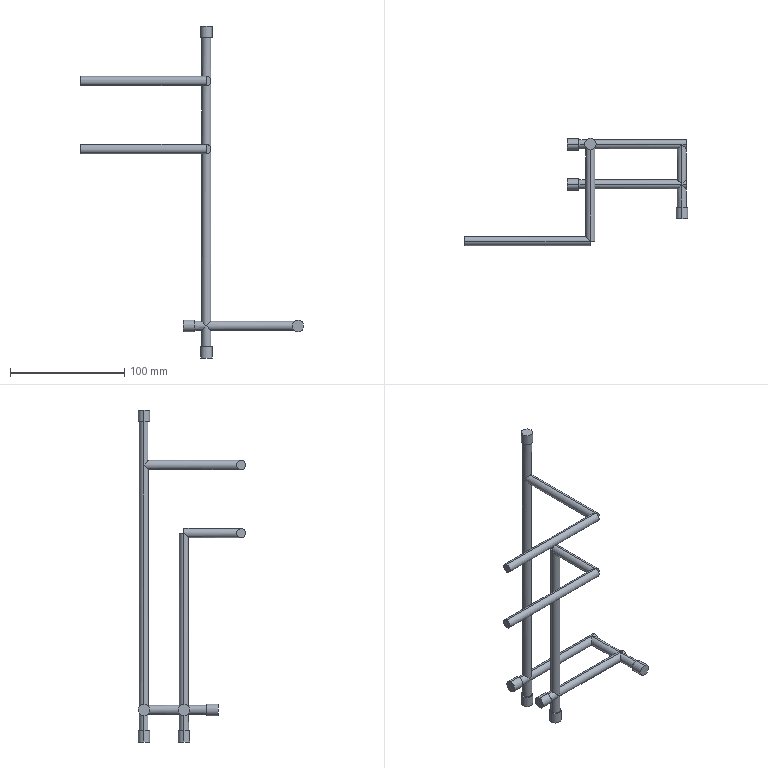Part | STEP file | 1 solid | 68 faces | box 195 x 94 x 290 mm | volume 55392 mm3 | cylinder 46 | plane 22 | commonest cylinder face diameters 8 x34 10 x12